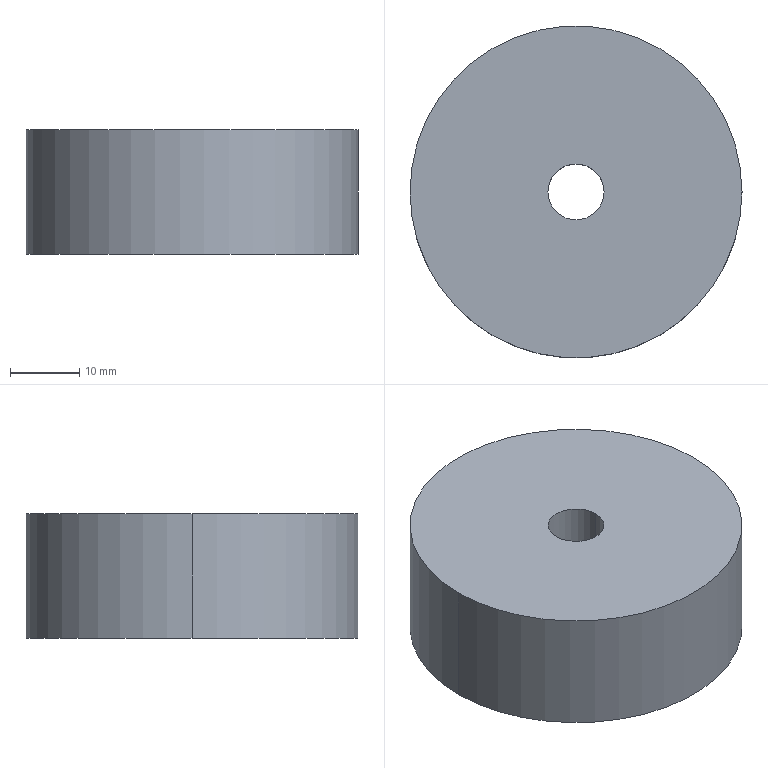Part | SolidWorks | features Extrusion 1 | 1 solid | 6 faces | box 48 x 48 x 18 mm | volume 31644 mm3 | cylinder 4 | plane 2 | commonest cylinder face diameters 8.1 x2 48 x2
STEP:
#1=CARTESIAN_POINT('',(-4.05,0.,18.));
#2=VERTEX_POINT('',#1);
#3=CARTESIAN_POINT('',(4.05,0.,18.));
#4=VERTEX_POINT('',#3);
#5=CARTESIAN_POINT('',(0.,0.,18.));
#6=DIRECTION('',(0.,0.,1.));
#7=DIRECTION('',(1.,0.,0.));
#8=AXIS2_PLACEMENT_3D('',#5,#6,#7);
#9=CIRCLE('',#8,4.05);
#10=EDGE_CURVE('',#2,#4,#9,.T.);
#11=ORIENTED_EDGE('',*,*,#10,.T.);
#12=CARTESIAN_POINT('',(4.05,0.,0.));
#13=VERTEX_POINT('',#12);
#14=CARTESIAN_POINT('',(4.05,0.,18.));
#15=DIRECTION('',(0.,0.,-1.));
#16=VECTOR('',#15,1000.);
#17=LINE('',#14,#16);
#18=EDGE_CURVE('',#4,#13,#17,.T.);
#19=ORIENTED_EDGE('',*,*,#18,.T.);
#20=CARTESIAN_POINT('',(-4.05,0.,0.));
#21=VERTEX_POINT('',#20);
#22=CARTESIAN_POINT('',(0.,0.,0.));
#23=DIRECTION('',(0.,0.,1.));
#24=DIRECTION('',(1.,0.,0.));
#25=AXIS2_PLACEMENT_3D('',#22,#23,#24);
#26=CIRCLE('',#25,4.05);
#27=EDGE_CURVE('',#21,#13,#26,.T.);
#28=ORIENTED_EDGE('',*,*,#27,.F.);
#29=CARTESIAN_POINT('',(-4.05,0.,18.));
#30=DIRECTION('',(0.,0.,-1.));
#31=VECTOR('',#30,1000.);
#32=LINE('',#29,#31);
#33=EDGE_CURVE('',#2,#21,#32,.T.);
#34=ORIENTED_EDGE('',*,*,#33,.F.);
#35=EDGE_LOOP('',(#11,#19,#28,#34));
#36=FACE_OUTER_BOUND('',#35,.T.);
#37=CARTESIAN_POINT('',(0.,0.,18.));
#38=DIRECTION('',(0.,0.,-1.));
#39=DIRECTION('',(-1.,0.,0.));
#40=AXIS2_PLACEMENT_3D('',#37,#38,#39);
#41=CYLINDRICAL_SURFACE('',#40,4.05);
#42=ADVANCED_FACE('',(#36),#41,.F.);
#43=CARTESIAN_POINT('',(24.,0.,18.));
#44=VERTEX_POINT('',#43);
#45=CARTESIAN_POINT('',(-24.,0.,18.));
#46=VERTEX_POINT('',#45);
#47=CARTESIAN_POINT('',(0.,0.,18.));
#48=DIRECTION('',(0.,0.,1.));
#49=DIRECTION('',(1.,0.,0.));
#50=AXIS2_PLACEMENT_3D('',#47,#48,#49);
#51=CIRCLE('',#50,24.);
#52=EDGE_CURVE('',#44,#46,#51,.T.);
#53=ORIENTED_EDGE('',*,*,#52,.F.);
#54=CARTESIAN_POINT('',(24.,0.,0.));
#55=VERTEX_POINT('',#54);
#56=CARTESIAN_POINT('',(24.,0.,18.));
#57=DIRECTION('',(0.,0.,-1.));
#58=VECTOR('',#57,1000.);
#59=LINE('',#56,#58);
#60=EDGE_CURVE('',#44,#55,#59,.T.);
#61=ORIENTED_EDGE('',*,*,#60,.T.);
#62=CARTESIAN_POINT('',(-24.,0.,0.));
#63=VERTEX_POINT('',#62);
#64=CARTESIAN_POINT('',(0.,0.,0.));
#65=DIRECTION('',(0.,0.,1.));
#66=DIRECTION('',(1.,0.,0.));
#67=AXIS2_PLACEMENT_3D('',#64,#65,#66);
#68=CIRCLE('',#67,24.);
#69=EDGE_CURVE('',#55,#63,#68,.T.);
#70=ORIENTED_EDGE('',*,*,#69,.T.);
#71=CARTESIAN_POINT('',(-24.,0.,18.));
#72=DIRECTION('',(0.,0.,-1.));
#73=VECTOR('',#72,1000.);
#74=LINE('',#71,#73);
#75=EDGE_CURVE('',#46,#63,#74,.T.);
#76=ORIENTED_EDGE('',*,*,#75,.F.);
#77=EDGE_LOOP('',(#53,#61,#70,#76));
#78=FACE_OUTER_BOUND('',#77,.T.);
#79=CARTESIAN_POINT('',(0.,0.,18.));
#80=DIRECTION('',(0.,0.,-1.));
#81=DIRECTION('',(-1.,0.,0.));
#82=AXIS2_PLACEMENT_3D('',#79,#80,#81);
#83=CYLINDRICAL_SURFACE('',#82,24.);
#84=ADVANCED_FACE('',(#78),#83,.T.);
#85=CARTESIAN_POINT('',(0.,0.,18.));
#86=DIRECTION('',(0.,0.,1.));
#87=DIRECTION('',(1.,0.,0.));
#88=AXIS2_PLACEMENT_3D('',#85,#86,#87);
#89=CIRCLE('',#88,24.);
#90=EDGE_CURVE('',#46,#44,#89,.T.);
#91=ORIENTED_EDGE('',*,*,#90,.T.);
#92=ORIENTED_EDGE('',*,*,#52,.T.);
#93=EDGE_LOOP('',(#91,#92));
#94=FACE_OUTER_BOUND('',#93,.T.);
#95=ORIENTED_EDGE('',*,*,#10,.F.);
#96=CARTESIAN_POINT('',(0.,0.,18.));
#97=DIRECTION('',(0.,0.,1.));
#98=DIRECTION('',(1.,0.,0.));
#99=AXIS2_PLACEMENT_3D('',#96,#97,#98);
#100=CIRCLE('',#99,4.05);
#101=EDGE_CURVE('',#4,#2,#100,.T.);
#102=ORIENTED_EDGE('',*,*,#101,.F.);
#103=EDGE_LOOP('',(#95,#102));
#104=FACE_BOUND('',#103,.T.);
#105=CARTESIAN_POINT('',(0.,0.,18.));
#106=DIRECTION('',(0.,0.,1.));
#107=DIRECTION('',(1.,0.,0.));
#108=AXIS2_PLACEMENT_3D('',#105,#106,#107);
#109=PLANE('',#108);
#110=ADVANCED_FACE('',(#94,#104),#109,.T.);
#111=CARTESIAN_POINT('',(0.,0.,0.));
#112=DIRECTION('',(0.,0.,1.));
#113=DIRECTION('',(1.,0.,0.));
#114=AXIS2_PLACEMENT_3D('',#111,#112,#113);
#115=CIRCLE('',#114,24.);
#116=EDGE_CURVE('',#63,#55,#115,.T.);
#117=ORIENTED_EDGE('',*,*,#116,.F.);
#118=ORIENTED_EDGE('',*,*,#69,.F.);
#119=EDGE_LOOP('',(#117,#118));
#120=FACE_OUTER_BOUND('',#119,.T.);
#121=ORIENTED_EDGE('',*,*,#27,.T.);
#122=CARTESIAN_POINT('',(0.,0.,0.));
#123=DIRECTION('',(0.,0.,1.));
#124=DIRECTION('',(1.,0.,0.));
#125=AXIS2_PLACEMENT_3D('',#122,#123,#124);
#126=CIRCLE('',#125,4.05);
#127=EDGE_CURVE('',#13,#21,#126,.T.);
#128=ORIENTED_EDGE('',*,*,#127,.T.);
#129=EDGE_LOOP('',(#121,#128));
#130=FACE_BOUND('',#129,.T.);
#131=CARTESIAN_POINT('',(0.,0.,0.));
#132=DIRECTION('',(0.,0.,1.));
#133=DIRECTION('',(1.,0.,0.));
#134=AXIS2_PLACEMENT_3D('',#131,#132,#133);
#135=PLANE('',#134);
#136=ADVANCED_FACE('',(#120,#130),#135,.F.);
#137=ORIENTED_EDGE('',*,*,#60,.F.);
#138=ORIENTED_EDGE('',*,*,#90,.F.);
#139=ORIENTED_EDGE('',*,*,#75,.T.);
#140=ORIENTED_EDGE('',*,*,#116,.T.);
#141=EDGE_LOOP('',(#137,#138,#139,#140));
#142=FACE_OUTER_BOUND('',#141,.T.);
#143=CARTESIAN_POINT('',(0.,0.,18.));
#144=DIRECTION('',(0.,0.,-1.));
#145=DIRECTION('',(-1.,0.,0.));
#146=AXIS2_PLACEMENT_3D('',#143,#144,#145);
#147=CYLINDRICAL_SURFACE('',#146,24.);
#148=ADVANCED_FACE('',(#142),#147,.T.);
#149=ORIENTED_EDGE('',*,*,#18,.F.);
#150=ORIENTED_EDGE('',*,*,#101,.T.);
#151=ORIENTED_EDGE('',*,*,#33,.T.);
#152=ORIENTED_EDGE('',*,*,#127,.F.);
#153=EDGE_LOOP('',(#149,#150,#151,#152));
#154=FACE_OUTER_BOUND('',#153,.T.);
#155=CARTESIAN_POINT('',(0.,0.,18.));
#156=DIRECTION('',(0.,0.,-1.));
#157=DIRECTION('',(-1.,0.,0.));
#158=AXIS2_PLACEMENT_3D('',#155,#156,#157);
#159=CYLINDRICAL_SURFACE('',#158,4.05);
#160=ADVANCED_FACE('',(#154),#159,.F.);
#161=CLOSED_SHELL('',(#42,#84,#110,#136,#148,#160));
#162=MANIFOLD_SOLID_BREP('',#161);
#163=CARTESIAN_POINT('',(0.,0.,0.));
#164=DIRECTION('',(0.,0.,1.));
#165=DIRECTION('',(1.,0.,0.));
#166=AXIS2_PLACEMENT_3D('',#163,#164,#165);
#167=(LENGTH_UNIT()NAMED_UNIT(*)SI_UNIT(.MILLI.,.METRE.));
#168=UNCERTAINTY_MEASURE_WITH_UNIT(LENGTH_MEASURE(0.00001),#167,'','');
#169=(NAMED_UNIT(*)PLANE_ANGLE_UNIT()SI_UNIT($,.RADIAN.));
#170=(NAMED_UNIT(*)SI_UNIT($,.STERADIAN.)SOLID_ANGLE_UNIT());
#171=(GEOMETRIC_REPRESENTATION_CONTEXT(3)GLOBAL_UNCERTAINTY_ASSIGNED_CONTEXT((#168))GLOBAL_UNIT_ASSIGNED_CONTEXT((#167,#169,#170))REPRESENTATION_CONTEXT('',''));
#172=ADVANCED_BREP_SHAPE_REPRESENTATION('',(#162,#166),#171);